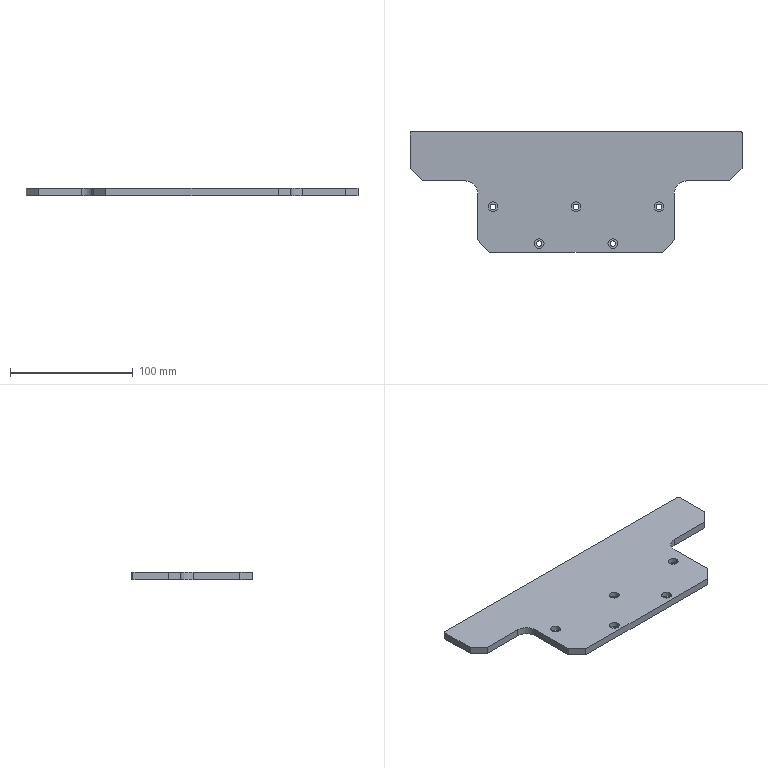Part | STEP file | 1 solid | 43 faces | box 270 x 98 x 6 mm | volume 118371 mm3 | cylinder 24 | plane 19 | commonest cylinder face diameters 4.5 x10 8 x10 2 x2 20 x2